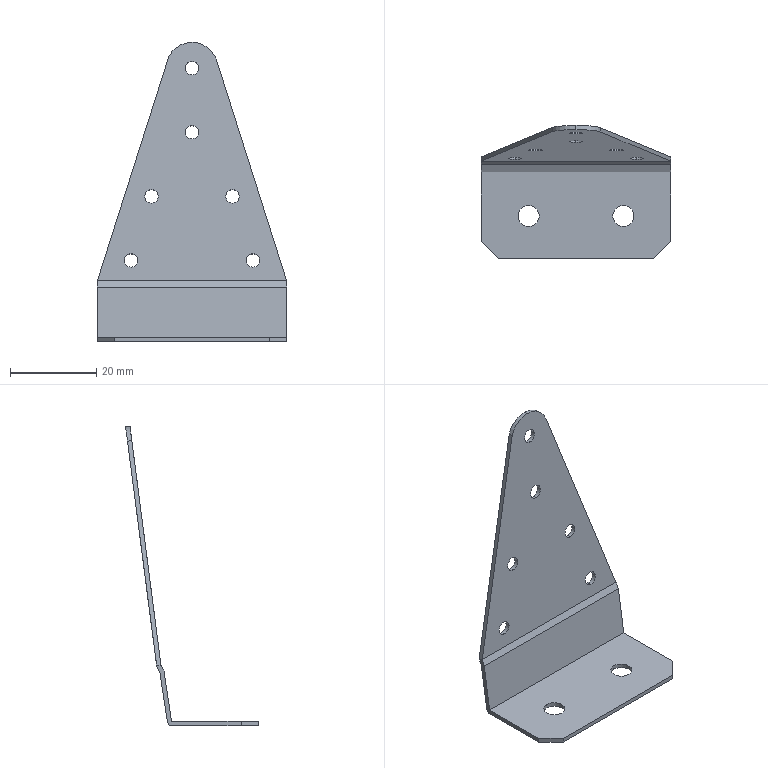Part | SolidWorks | features BaseBody 1 | 1 solid | 34 faces | box 44 x 30.796 x 69.44 mm | volume 2867 mm3 | cylinder 19 | plane 15 | commonest cylinder face diameters 3.2 x12 4.9 x4 12 x2 2 x1
STEP:
#1=CARTESIAN_POINT('',(-153.,101.05,-969.));
#2=VERTEX_POINT('',#1);
#3=CARTESIAN_POINT('',(-153.,105.95,-969.));
#4=VERTEX_POINT('',#3);
#5=CARTESIAN_POINT('',(-153.,103.5,-969.));
#6=DIRECTION('',(0.,0.,-1.));
#7=DIRECTION('',(0.,-1.,0.));
#8=AXIS2_PLACEMENT_3D('',#5,#6,#7);
#9=CIRCLE('',#8,2.45);
#10=EDGE_CURVE('',#2,#4,#9,.T.);
#11=ORIENTED_EDGE('',*,*,#10,.T.);
#12=CARTESIAN_POINT('',(-153.,105.95,-968.));
#13=VERTEX_POINT('',#12);
#14=CARTESIAN_POINT('',(-153.,105.95,-969.));
#15=DIRECTION('',(0.,0.,1.));
#16=VECTOR('',#15,1000.);
#17=LINE('',#14,#16);
#18=EDGE_CURVE('',#4,#13,#17,.T.);
#19=ORIENTED_EDGE('',*,*,#18,.T.);
#20=CARTESIAN_POINT('',(-153.,101.05,-968.));
#21=VERTEX_POINT('',#20);
#22=CARTESIAN_POINT('',(-153.,103.5,-968.));
#23=DIRECTION('',(0.,0.,1.));
#24=DIRECTION('',(0.,-1.,0.));
#25=AXIS2_PLACEMENT_3D('',#22,#23,#24);
#26=CIRCLE('',#25,2.45);
#27=EDGE_CURVE('',#13,#21,#26,.T.);
#28=ORIENTED_EDGE('',*,*,#27,.T.);
#29=CARTESIAN_POINT('',(-153.,101.05,-969.));
#30=DIRECTION('',(0.,0.,1.));
#31=VECTOR('',#30,1000.);
#32=LINE('',#29,#31);
#33=EDGE_CURVE('',#2,#21,#32,.T.);
#34=ORIENTED_EDGE('',*,*,#33,.F.);
#35=EDGE_LOOP('',(#11,#19,#28,#34));
#36=FACE_OUTER_BOUND('',#35,.T.);
#37=CARTESIAN_POINT('',(-153.,103.5,-969.));
#38=DIRECTION('',(0.,0.,1.));
#39=DIRECTION('',(0.,-1.,0.));
#40=AXIS2_PLACEMENT_3D('',#37,#38,#39);
#41=CYLINDRICAL_SURFACE('',#40,2.45);
#42=ADVANCED_FACE('',(#36),#41,.F.);
#43=CARTESIAN_POINT('',(-131.,101.05,-969.));
#44=VERTEX_POINT('',#43);
#45=CARTESIAN_POINT('',(-131.,105.95,-969.));
#46=VERTEX_POINT('',#45);
#47=CARTESIAN_POINT('',(-131.,103.5,-969.));
#48=DIRECTION('',(0.,0.,-1.));
#49=DIRECTION('',(0.,-1.,0.));
#50=AXIS2_PLACEMENT_3D('',#47,#48,#49);
#51=CIRCLE('',#50,2.45);
#52=EDGE_CURVE('',#44,#46,#51,.T.);
#53=ORIENTED_EDGE('',*,*,#52,.T.);
#54=CARTESIAN_POINT('',(-131.,105.95,-968.));
#55=VERTEX_POINT('',#54);
#56=CARTESIAN_POINT('',(-131.,105.95,-969.));
#57=DIRECTION('',(0.,0.,1.));
#58=VECTOR('',#57,1000.);
#59=LINE('',#56,#58);
#60=EDGE_CURVE('',#46,#55,#59,.T.);
#61=ORIENTED_EDGE('',*,*,#60,.T.);
#62=CARTESIAN_POINT('',(-131.,101.05,-968.));
#63=VERTEX_POINT('',#62);
#64=CARTESIAN_POINT('',(-131.,103.5,-968.));
#65=DIRECTION('',(0.,0.,1.));
#66=DIRECTION('',(0.,-1.,0.));
#67=AXIS2_PLACEMENT_3D('',#64,#65,#66);
#68=CIRCLE('',#67,2.45);
#69=EDGE_CURVE('',#55,#63,#68,.T.);
#70=ORIENTED_EDGE('',*,*,#69,.T.);
#71=CARTESIAN_POINT('',(-131.,101.05,-969.));
#72=DIRECTION('',(0.,0.,1.));
#73=VECTOR('',#72,1000.);
#74=LINE('',#71,#73);
#75=EDGE_CURVE('',#44,#63,#74,.T.);
#76=ORIENTED_EDGE('',*,*,#75,.F.);
#77=EDGE_LOOP('',(#53,#61,#70,#76));
#78=FACE_OUTER_BOUND('',#77,.T.);
#79=CARTESIAN_POINT('',(-131.,103.5,-969.));
#80=DIRECTION('',(0.,0.,1.));
#81=DIRECTION('',(0.,-1.,0.));
#82=AXIS2_PLACEMENT_3D('',#79,#80,#81);
#83=CYLINDRICAL_SURFACE('',#82,2.45);
#84=ADVANCED_FACE('',(#78),#83,.F.);
#85=CARTESIAN_POINT('',(-156.144,117.061,-948.549));
#86=VERTEX_POINT('',#85);
#87=CARTESIAN_POINT('',(-156.144,116.649,-951.723));
#88=VERTEX_POINT('',#87);
#89=CARTESIAN_POINT('',(-156.144,116.855,-950.136));
#90=DIRECTION('',(0.,-0.9917,0.1287));
#91=DIRECTION('',(0.,0.1287,0.9917));
#92=AXIS2_PLACEMENT_3D('',#89,#90,#91);
#93=CIRCLE('',#92,1.6);
#94=EDGE_CURVE('',#86,#88,#93,.T.);
#95=ORIENTED_EDGE('',*,*,#94,.T.);
#96=CARTESIAN_POINT('',(-156.144,117.641,-951.851));
#97=VERTEX_POINT('',#96);
#98=CARTESIAN_POINT('',(-156.144,116.649,-951.723));
#99=DIRECTION('',(0.,0.9917,-0.1287));
#100=VECTOR('',#99,1000.);
#101=LINE('',#98,#100);
#102=EDGE_CURVE('',#88,#97,#101,.T.);
#103=ORIENTED_EDGE('',*,*,#102,.T.);
#104=CARTESIAN_POINT('',(-156.144,118.053,-948.678));
#105=VERTEX_POINT('',#104);
#106=CARTESIAN_POINT('',(-156.144,117.847,-950.265));
#107=DIRECTION('',(0.,0.9917,-0.1287));
#108=DIRECTION('',(0.,0.1287,0.9917));
#109=AXIS2_PLACEMENT_3D('',#106,#107,#108);
#110=CIRCLE('',#109,1.6);
#111=EDGE_CURVE('',#97,#105,#110,.T.);
#112=ORIENTED_EDGE('',*,*,#111,.T.);
#113=CARTESIAN_POINT('',(-156.144,117.061,-948.549));
#114=DIRECTION('',(0.,0.9917,-0.1287));
#115=VECTOR('',#114,1000.);
#116=LINE('',#113,#115);
#117=EDGE_CURVE('',#86,#105,#116,.T.);
#118=ORIENTED_EDGE('',*,*,#117,.F.);
#119=EDGE_LOOP('',(#95,#103,#112,#118));
#120=FACE_OUTER_BOUND('',#119,.T.);
#121=CARTESIAN_POINT('',(-156.144,116.855,-950.136));
#122=DIRECTION('',(0.,0.9917,-0.1287));
#123=DIRECTION('',(0.,0.1287,0.9917));
#124=AXIS2_PLACEMENT_3D('',#121,#122,#123);
#125=CYLINDRICAL_SURFACE('',#124,1.6);
#126=ADVANCED_FACE('',(#120),#125,.F.);
#127=CARTESIAN_POINT('',(-151.404,118.991,-933.674));
#128=VERTEX_POINT('',#127);
#129=CARTESIAN_POINT('',(-151.404,118.58,-936.847));
#130=VERTEX_POINT('',#129);
#131=CARTESIAN_POINT('',(-151.404,118.786,-935.261));
#132=DIRECTION('',(0.,-0.9917,0.1287));
#133=DIRECTION('',(0.,0.1287,0.9917));
#134=AXIS2_PLACEMENT_3D('',#131,#132,#133);
#135=CIRCLE('',#134,1.6);
#136=EDGE_CURVE('',#128,#130,#135,.T.);
#137=ORIENTED_EDGE('',*,*,#136,.T.);
#138=CARTESIAN_POINT('',(-151.404,119.571,-936.976));
#139=VERTEX_POINT('',#138);
#140=CARTESIAN_POINT('',(-151.404,118.58,-936.847));
#141=DIRECTION('',(0.,0.9917,-0.1287));
#142=VECTOR('',#141,1000.);
#143=LINE('',#140,#142);
#144=EDGE_CURVE('',#130,#139,#143,.T.);
#145=ORIENTED_EDGE('',*,*,#144,.T.);
#146=CARTESIAN_POINT('',(-151.404,119.983,-933.803));
#147=VERTEX_POINT('',#146);
#148=CARTESIAN_POINT('',(-151.404,119.777,-935.389));
#149=DIRECTION('',(0.,0.9917,-0.1287));
#150=DIRECTION('',(0.,0.1287,0.9917));
#151=AXIS2_PLACEMENT_3D('',#148,#149,#150);
#152=CIRCLE('',#151,1.6);
#153=EDGE_CURVE('',#139,#147,#152,.T.);
#154=ORIENTED_EDGE('',*,*,#153,.T.);
#155=CARTESIAN_POINT('',(-151.404,118.991,-933.674));
#156=DIRECTION('',(0.,0.9917,-0.1287));
#157=VECTOR('',#156,1000.);
#158=LINE('',#155,#157);
#159=EDGE_CURVE('',#128,#147,#158,.T.);
#160=ORIENTED_EDGE('',*,*,#159,.F.);
#161=EDGE_LOOP('',(#137,#145,#154,#160));
#162=FACE_OUTER_BOUND('',#161,.T.);
#163=CARTESIAN_POINT('',(-151.404,118.786,-935.261));
#164=DIRECTION('',(0.,0.9917,-0.1287));
#165=DIRECTION('',(0.,0.1287,0.9917));
#166=AXIS2_PLACEMENT_3D('',#163,#164,#165);
#167=CYLINDRICAL_SURFACE('',#166,1.6);
#168=ADVANCED_FACE('',(#162),#167,.F.);
#169=CARTESIAN_POINT('',(-142.,122.852,-903.924));
#170=VERTEX_POINT('',#169);
#171=CARTESIAN_POINT('',(-142.,122.44,-907.097));
#172=VERTEX_POINT('',#171);
#173=CARTESIAN_POINT('',(-142.,122.646,-905.51));
#174=DIRECTION('',(0.,-0.9917,0.1287));
#175=DIRECTION('',(0.,0.1287,0.9917));
#176=AXIS2_PLACEMENT_3D('',#173,#174,#175);
#177=CIRCLE('',#176,1.6);
#178=EDGE_CURVE('',#170,#172,#177,.T.);
#179=ORIENTED_EDGE('',*,*,#178,.T.);
#180=CARTESIAN_POINT('',(-142.,123.432,-907.226));
#181=VERTEX_POINT('',#180);
#182=CARTESIAN_POINT('',(-142.,122.44,-907.097));
#183=DIRECTION('',(0.,0.9917,-0.1287));
#184=VECTOR('',#183,1000.);
#185=LINE('',#182,#184);
#186=EDGE_CURVE('',#172,#181,#185,.T.);
#187=ORIENTED_EDGE('',*,*,#186,.T.);
#188=CARTESIAN_POINT('',(-142.,123.844,-904.052));
#189=VERTEX_POINT('',#188);
#190=CARTESIAN_POINT('',(-142.,123.638,-905.639));
#191=DIRECTION('',(0.,0.9917,-0.1287));
#192=DIRECTION('',(0.,0.1287,0.9917));
#193=AXIS2_PLACEMENT_3D('',#190,#191,#192);
#194=CIRCLE('',#193,1.6);
#195=EDGE_CURVE('',#181,#189,#194,.T.);
#196=ORIENTED_EDGE('',*,*,#195,.T.);
#197=CARTESIAN_POINT('',(-142.,122.852,-903.924));
#198=DIRECTION('',(0.,0.9917,-0.1287));
#199=VECTOR('',#198,1000.);
#200=LINE('',#197,#199);
#201=EDGE_CURVE('',#170,#189,#200,.T.);
#202=ORIENTED_EDGE('',*,*,#201,.F.);
#203=EDGE_LOOP('',(#179,#187,#196,#202));
#204=FACE_OUTER_BOUND('',#203,.T.);
#205=CARTESIAN_POINT('',(-142.,122.646,-905.51));
#206=DIRECTION('',(0.,0.9917,-0.1287));
#207=DIRECTION('',(0.,0.1287,0.9917));
#208=AXIS2_PLACEMENT_3D('',#205,#206,#207);
#209=CYLINDRICAL_SURFACE('',#208,1.6);
#210=ADVANCED_FACE('',(#204),#209,.F.);
#211=CARTESIAN_POINT('',(-142.,120.922,-918.799));
#212=VERTEX_POINT('',#211);
#213=CARTESIAN_POINT('',(-142.,120.51,-921.972));
#214=VERTEX_POINT('',#213);
#215=CARTESIAN_POINT('',(-142.,120.716,-920.386));
#216=DIRECTION('',(0.,-0.9917,0.1287));
#217=DIRECTION('',(0.,0.1287,0.9917));
#218=AXIS2_PLACEMENT_3D('',#215,#216,#217);
#219=CIRCLE('',#218,1.6);
#220=EDGE_CURVE('',#212,#214,#219,.T.);
#221=ORIENTED_EDGE('',*,*,#220,.T.);
#222=CARTESIAN_POINT('',(-142.,121.502,-922.101));
#223=VERTEX_POINT('',#222);
#224=CARTESIAN_POINT('',(-142.,120.51,-921.972));
#225=DIRECTION('',(0.,0.9917,-0.1287));
#226=VECTOR('',#225,1000.);
#227=LINE('',#224,#226);
#228=EDGE_CURVE('',#214,#223,#227,.T.);
#229=ORIENTED_EDGE('',*,*,#228,.T.);
#230=CARTESIAN_POINT('',(-142.,121.913,-918.928));
#231=VERTEX_POINT('',#230);
#232=CARTESIAN_POINT('',(-142.,121.708,-920.514));
#233=DIRECTION('',(0.,0.9917,-0.1287));
#234=DIRECTION('',(0.,0.1287,0.9917));
#235=AXIS2_PLACEMENT_3D('',#232,#233,#234);
#236=CIRCLE('',#235,1.6);
#237=EDGE_CURVE('',#223,#231,#236,.T.);
#238=ORIENTED_EDGE('',*,*,#237,.T.);
#239=CARTESIAN_POINT('',(-142.,120.922,-918.799));
#240=DIRECTION('',(0.,0.9917,-0.1287));
#241=VECTOR('',#240,1000.);
#242=LINE('',#239,#241);
#243=EDGE_CURVE('',#212,#231,#242,.T.);
#244=ORIENTED_EDGE('',*,*,#243,.F.);
#245=EDGE_LOOP('',(#221,#229,#238,#244));
#246=FACE_OUTER_BOUND('',#245,.T.);
#247=CARTESIAN_POINT('',(-142.,120.716,-920.386));
#248=DIRECTION('',(0.,0.9917,-0.1287));
#249=DIRECTION('',(0.,0.1287,0.9917));
#250=AXIS2_PLACEMENT_3D('',#247,#248,#249);
#251=CYLINDRICAL_SURFACE('',#250,1.6);
#252=ADVANCED_FACE('',(#246),#251,.F.);
#253=CARTESIAN_POINT('',(-132.596,118.991,-933.674));
#254=VERTEX_POINT('',#253);
#255=CARTESIAN_POINT('',(-132.596,118.58,-936.847));
#256=VERTEX_POINT('',#255);
#257=CARTESIAN_POINT('',(-132.596,118.786,-935.261));
#258=DIRECTION('',(0.,-0.9917,0.1287));
#259=DIRECTION('',(0.,0.1287,0.9917));
#260=AXIS2_PLACEMENT_3D('',#257,#258,#259);
#261=CIRCLE('',#260,1.6);
#262=EDGE_CURVE('',#254,#256,#261,.T.);
#263=ORIENTED_EDGE('',*,*,#262,.T.);
#264=CARTESIAN_POINT('',(-132.596,119.571,-936.976));
#265=VERTEX_POINT('',#264);
#266=CARTESIAN_POINT('',(-132.596,118.58,-936.847));
#267=DIRECTION('',(0.,0.9917,-0.1287));
#268=VECTOR('',#267,1000.);
#269=LINE('',#266,#268);
#270=EDGE_CURVE('',#256,#265,#269,.T.);
#271=ORIENTED_EDGE('',*,*,#270,.T.);
#272=CARTESIAN_POINT('',(-132.596,119.983,-933.803));
#273=VERTEX_POINT('',#272);
#274=CARTESIAN_POINT('',(-132.596,119.777,-935.389));
#275=DIRECTION('',(0.,0.9917,-0.1287));
#276=DIRECTION('',(0.,0.1287,0.9917));
#277=AXIS2_PLACEMENT_3D('',#274,#275,#276);
#278=CIRCLE('',#277,1.6);
#279=EDGE_CURVE('',#265,#273,#278,.T.);
#280=ORIENTED_EDGE('',*,*,#279,.T.);
#281=CARTESIAN_POINT('',(-132.596,118.991,-933.674));
#282=DIRECTION('',(0.,0.9917,-0.1287));
#283=VECTOR('',#282,1000.);
#284=LINE('',#281,#283);
#285=EDGE_CURVE('',#254,#273,#284,.T.);
#286=ORIENTED_EDGE('',*,*,#285,.F.);
#287=EDGE_LOOP('',(#263,#271,#280,#286));
#288=FACE_OUTER_BOUND('',#287,.T.);
#289=CARTESIAN_POINT('',(-132.596,118.786,-935.261));
#290=DIRECTION('',(0.,0.9917,-0.1287));
#291=DIRECTION('',(0.,0.1287,0.9917));
#292=AXIS2_PLACEMENT_3D('',#289,#290,#291);
#293=CYLINDRICAL_SURFACE('',#292,1.6);
#294=ADVANCED_FACE('',(#288),#293,.F.);
#295=CARTESIAN_POINT('',(-127.856,117.061,-948.549));
#296=VERTEX_POINT('',#295);
#297=CARTESIAN_POINT('',(-127.856,116.649,-951.723));
#298=VERTEX_POINT('',#297);
#299=CARTESIAN_POINT('',(-127.856,116.855,-950.136));
#300=DIRECTION('',(0.,-0.9917,0.1287));
#301=DIRECTION('',(0.,0.1287,0.9917));
#302=AXIS2_PLACEMENT_3D('',#299,#300,#301);
#303=CIRCLE('',#302,1.6);
#304=EDGE_CURVE('',#296,#298,#303,.T.);
#305=ORIENTED_EDGE('',*,*,#304,.T.);
#306=CARTESIAN_POINT('',(-127.856,117.641,-951.851));
#307=VERTEX_POINT('',#306);
#308=CARTESIAN_POINT('',(-127.856,116.649,-951.723));
#309=DIRECTION('',(0.,0.9917,-0.1287));
#310=VECTOR('',#309,1000.);
#311=LINE('',#308,#310);
#312=EDGE_CURVE('',#298,#307,#311,.T.);
#313=ORIENTED_EDGE('',*,*,#312,.T.);
#314=CARTESIAN_POINT('',(-127.856,118.053,-948.678));
#315=VERTEX_POINT('',#314);
#316=CARTESIAN_POINT('',(-127.856,117.847,-950.265));
#317=DIRECTION('',(0.,0.9917,-0.1287));
#318=DIRECTION('',(0.,0.1287,0.9917));
#319=AXIS2_PLACEMENT_3D('',#316,#317,#318);
#320=CIRCLE('',#319,1.6);
#321=EDGE_CURVE('',#307,#315,#320,.T.);
#322=ORIENTED_EDGE('',*,*,#321,.T.);
#323=CARTESIAN_POINT('',(-127.856,117.061,-948.549));
#324=DIRECTION('',(0.,0.9917,-0.1287));
#325=VECTOR('',#324,1000.);
#326=LINE('',#323,#325);
#327=EDGE_CURVE('',#296,#315,#326,.T.);
#328=ORIENTED_EDGE('',*,*,#327,.F.);
#329=EDGE_LOOP('',(#305,#313,#322,#328));
#330=FACE_OUTER_BOUND('',#329,.T.);
#331=CARTESIAN_POINT('',(-127.856,116.855,-950.136));
#332=DIRECTION('',(0.,0.9917,-0.1287));
#333=DIRECTION('',(0.,0.1287,0.9917));
#334=AXIS2_PLACEMENT_3D('',#331,#332,#333);
#335=CYLINDRICAL_SURFACE('',#334,1.6);
#336=ADVANCED_FACE('',(#330),#335,.F.);
#337=CARTESIAN_POINT('',(-147.37,122.99,-902.856));
#338=VERTEX_POINT('',#337);
#339=CARTESIAN_POINT('',(-142.,123.418,-899.56));
#340=VERTEX_POINT('',#339);
#341=CARTESIAN_POINT('',(-142.,122.646,-905.51));
#342=DIRECTION('',(0.,0.9917,-0.1287));
#343=DIRECTION('',(0.,0.1287,0.9917));
#344=AXIS2_PLACEMENT_3D('',#341,#342,#343);
#345=CIRCLE('',#344,6.);
#346=EDGE_CURVE('',#338,#340,#345,.T.);
#347=ORIENTED_EDGE('',*,*,#346,.T.);
#348=CARTESIAN_POINT('',(-142.,124.41,-899.689));
#349=VERTEX_POINT('',#348);
#350=CARTESIAN_POINT('',(-142.,123.418,-899.56));
#351=DIRECTION('',(0.,0.9917,-0.1287));
#352=VECTOR('',#351,1000.);
#353=LINE('',#350,#352);
#354=EDGE_CURVE('',#340,#349,#353,.T.);
#355=ORIENTED_EDGE('',*,*,#354,.T.);
#356=CARTESIAN_POINT('',(-147.37,123.982,-902.985));
#357=VERTEX_POINT('',#356);
#358=CARTESIAN_POINT('',(-142.,123.638,-905.639));
#359=DIRECTION('',(0.,-0.9917,0.1287));
#360=DIRECTION('',(0.,0.1287,0.9917));
#361=AXIS2_PLACEMENT_3D('',#358,#359,#360);
#362=CIRCLE('',#361,6.);
#363=EDGE_CURVE('',#349,#357,#362,.T.);
#364=ORIENTED_EDGE('',*,*,#363,.T.);
#365=CARTESIAN_POINT('',(-147.37,123.486,-902.921));
#366=DIRECTION('',(0.,0.9917,-0.1287));
#367=VECTOR('',#366,1000.);
#368=LINE('',#365,#367);
#369=EDGE_CURVE('',#338,#357,#368,.T.);
#370=ORIENTED_EDGE('',*,*,#369,.F.);
#371=EDGE_LOOP('',(#347,#355,#364,#370));
#372=FACE_OUTER_BOUND('',#371,.T.);
#373=CARTESIAN_POINT('',(-142.,122.646,-905.51));
#374=DIRECTION('',(0.,0.9917,-0.1287));
#375=DIRECTION('',(0.,0.1287,0.9917));
#376=AXIS2_PLACEMENT_3D('',#373,#374,#375);
#377=CYLINDRICAL_SURFACE('',#376,6.);
#378=ADVANCED_FACE('',(#372),#377,.T.);
#379=ORIENTED_EDGE('',*,*,#18,.F.);
#380=CARTESIAN_POINT('',(-153.,103.5,-969.));
#381=DIRECTION('',(0.,0.,-1.));
#382=DIRECTION('',(0.,-1.,0.));
#383=AXIS2_PLACEMENT_3D('',#380,#381,#382);
#384=CIRCLE('',#383,2.45);
#385=EDGE_CURVE('',#4,#2,#384,.T.);
#386=ORIENTED_EDGE('',*,*,#385,.T.);
#387=ORIENTED_EDGE('',*,*,#33,.T.);
#388=CARTESIAN_POINT('',(-153.,103.5,-968.));
#389=DIRECTION('',(0.,0.,1.));
#390=DIRECTION('',(0.,-1.,0.));
#391=AXIS2_PLACEMENT_3D('',#388,#389,#390);
#392=CIRCLE('',#391,2.45);
#393=EDGE_CURVE('',#21,#13,#392,.T.);
#394=ORIENTED_EDGE('',*,*,#393,.T.);
#395=EDGE_LOOP('',(#379,#386,#387,#394));
#396=FACE_OUTER_BOUND('',#395,.T.);
#397=CARTESIAN_POINT('',(-153.,103.5,-969.));
#398=DIRECTION('',(0.,0.,1.));
#399=DIRECTION('',(0.,-1.,0.));
#400=AXIS2_PLACEMENT_3D('',#397,#398,#399);
#401=CYLINDRICAL_SURFACE('',#400,2.45);
#402=ADVANCED_FACE('',(#396),#401,.F.);
#403=CARTESIAN_POINT('',(-131.,103.5,-968.));
#404=DIRECTION('',(0.,0.,1.));
#405=DIRECTION('',(0.,-1.,0.));
#406=AXIS2_PLACEMENT_3D('',#403,#404,#405);
#407=CIRCLE('',#406,2.45);
#408=EDGE_CURVE('',#63,#55,#407,.T.);
#409=ORIENTED_EDGE('',*,*,#408,.F.);
#410=ORIENTED_EDGE('',*,*,#69,.F.);
#411=EDGE_LOOP('',(#409,#410));
#412=FACE_BOUND('',#411,.T.);
#413=ORIENTED_EDGE('',*,*,#393,.F.);
#414=ORIENTED_EDGE('',*,*,#27,.F.);
#415=EDGE_LOOP('',(#413,#414));
#416=FACE_BOUND('',#415,.T.);
#417=CARTESIAN_POINT('',(-160.,93.614,-968.));
#418=VERTEX_POINT('',#417);
#419=CARTESIAN_POINT('',(-164.,97.614,-968.));
#420=VERTEX_POINT('',#419);
#421=CARTESIAN_POINT('',(-164.,97.614,-968.));
#422=DIRECTION('',(-0.7071,0.7071,0.));
#423=VECTOR('',#422,1000.);
#424=LINE('',#421,#423);
#425=EDGE_CURVE('',#418,#420,#424,.T.);
#426=ORIENTED_EDGE('',*,*,#425,.F.);
#427=CARTESIAN_POINT('',(-124.,93.614,-968.));
#428=VERTEX_POINT('',#427);
#429=CARTESIAN_POINT('',(-142.,93.614,-968.));
#430=DIRECTION('',(-1.,0.,0.));
#431=VECTOR('',#430,1000.);
#432=LINE('',#429,#431);
#433=EDGE_CURVE('',#428,#418,#432,.T.);
#434=ORIENTED_EDGE('',*,*,#433,.F.);
#435=CARTESIAN_POINT('',(-120.,97.614,-968.));
#436=VERTEX_POINT('',#435);
#437=CARTESIAN_POINT('',(-124.,93.614,-968.));
#438=DIRECTION('',(-0.7071,-0.7071,0.));
#439=VECTOR('',#438,1000.);
#440=LINE('',#437,#439);
#441=EDGE_CURVE('',#436,#428,#440,.T.);
#442=ORIENTED_EDGE('',*,*,#441,.F.);
#443=CARTESIAN_POINT('',(-120.,113.753,-968.));
#444=VERTEX_POINT('',#443);
#445=CARTESIAN_POINT('',(-120.,103.684,-968.));
#446=DIRECTION('',(0.,-1.,0.));
#447=VECTOR('',#446,1000.);
#448=LINE('',#445,#447);
#449=EDGE_CURVE('',#444,#436,#448,.T.);
#450=ORIENTED_EDGE('',*,*,#449,.F.);
#451=CARTESIAN_POINT('',(-164.,113.753,-968.));
#452=VERTEX_POINT('',#451);
#453=CARTESIAN_POINT('',(-142.,113.753,-968.));
#454=DIRECTION('',(1.,0.,0.));
#455=VECTOR('',#454,1000.);
#456=LINE('',#453,#455);
#457=EDGE_CURVE('',#452,#444,#456,.T.);
#458=ORIENTED_EDGE('',*,*,#457,.F.);
#459=CARTESIAN_POINT('',(-164.,103.684,-968.));
#460=DIRECTION('',(0.,1.,0.));
#461=VECTOR('',#460,1000.);
#462=LINE('',#459,#461);
#463=EDGE_CURVE('',#420,#452,#462,.T.);
#464=ORIENTED_EDGE('',*,*,#463,.F.);
#465=EDGE_LOOP('',(#426,#434,#442,#450,#458,#464));
#466=FACE_OUTER_BOUND('',#465,.T.);
#467=CARTESIAN_POINT('',(-120.,93.614,-968.));
#468=DIRECTION('',(0.,0.,-1.));
#469=DIRECTION('',(-1.,0.,0.));
#470=AXIS2_PLACEMENT_3D('',#467,#468,#469);
#471=PLANE('',#470);
#472=ADVANCED_FACE('',(#412,#416,#466),#471,.F.);
#473=ORIENTED_EDGE('',*,*,#52,.F.);
#474=CARTESIAN_POINT('',(-131.,103.5,-969.));
#475=DIRECTION('',(0.,0.,-1.));
#476=DIRECTION('',(0.,-1.,0.));
#477=AXIS2_PLACEMENT_3D('',#474,#475,#476);
#478=CIRCLE('',#477,2.45);
#479=EDGE_CURVE('',#46,#44,#478,.T.);
#480=ORIENTED_EDGE('',*,*,#479,.F.);
#481=EDGE_LOOP('',(#473,#480));
#482=FACE_BOUND('',#481,.T.);
#483=ORIENTED_EDGE('',*,*,#10,.F.);
#484=ORIENTED_EDGE('',*,*,#385,.F.);
#485=EDGE_LOOP('',(#483,#484));
#486=FACE_BOUND('',#485,.T.);
#487=CARTESIAN_POINT('',(-164.,97.614,-969.));
#488=VERTEX_POINT('',#487);
#489=CARTESIAN_POINT('',(-160.,93.614,-969.));
#490=VERTEX_POINT('',#489);
#491=CARTESIAN_POINT('',(-164.,97.614,-969.));
#492=DIRECTION('',(0.7071,-0.7071,0.));
#493=VECTOR('',#492,1000.);
#494=LINE('',#491,#493);
#495=EDGE_CURVE('',#488,#490,#494,.T.);
#496=ORIENTED_EDGE('',*,*,#495,.F.);
#497=CARTESIAN_POINT('',(-164.,113.753,-969.));
#498=VERTEX_POINT('',#497);
#499=CARTESIAN_POINT('',(-164.,103.684,-969.));
#500=DIRECTION('',(0.,-1.,0.));
#501=VECTOR('',#500,1000.);
#502=LINE('',#499,#501);
#503=EDGE_CURVE('',#498,#488,#502,.T.);
#504=ORIENTED_EDGE('',*,*,#503,.F.);
#505=CARTESIAN_POINT('',(-120.,113.753,-969.));
#506=VERTEX_POINT('',#505);
#507=CARTESIAN_POINT('',(-142.,113.753,-969.));
#508=DIRECTION('',(-1.,0.,0.));
#509=VECTOR('',#508,1000.);
#510=LINE('',#507,#509);
#511=EDGE_CURVE('',#506,#498,#510,.T.);
#512=ORIENTED_EDGE('',*,*,#511,.F.);
#513=CARTESIAN_POINT('',(-120.,97.614,-969.));
#514=VERTEX_POINT('',#513);
#515=CARTESIAN_POINT('',(-120.,103.684,-969.));
#516=DIRECTION('',(0.,1.,0.));
#517=VECTOR('',#516,1000.);
#518=LINE('',#515,#517);
#519=EDGE_CURVE('',#514,#506,#518,.T.);
#520=ORIENTED_EDGE('',*,*,#519,.F.);
#521=CARTESIAN_POINT('',(-124.,93.614,-969.));
#522=VERTEX_POINT('',#521);
#523=CARTESIAN_POINT('',(-124.,93.614,-969.));
#524=DIRECTION('',(0.7071,0.7071,0.));
#525=VECTOR('',#524,1000.);
#526=LINE('',#523,#525);
#527=EDGE_CURVE('',#522,#514,#526,.T.);
#528=ORIENTED_EDGE('',*,*,#527,.F.);
#529=CARTESIAN_POINT('',(-142.,93.614,-969.));
#530=DIRECTION('',(1.,0.,0.));
#531=VECTOR('',#530,1000.);
#532=LINE('',#529,#531);
#533=EDGE_CURVE('',#490,#522,#532,.T.);
#534=ORIENTED_EDGE('',*,*,#533,.F.);
#535=EDGE_LOOP('',(#496,#504,#512,#520,#528,#534));
#536=FACE_OUTER_BOUND('',#535,.T.);
#537=CARTESIAN_POINT('',(-164.,93.614,-969.));
#538=DIRECTION('',(0.,0.,1.));
#539=DIRECTION('',(1.,0.,0.));
#540=AXIS2_PLACEMENT_3D('',#537,#538,#539);
#541=PLANE('',#540);
#542=ADVANCED_FACE('',(#482,#486,#536),#541,.F.);
#543=ORIENTED_EDGE('',*,*,#60,.F.);
#544=ORIENTED_EDGE('',*,*,#479,.T.);
#545=ORIENTED_EDGE('',*,*,#75,.T.);
#546=ORIENTED_EDGE('',*,*,#408,.T.);
#547=EDGE_LOOP('',(#543,#544,#545,#546));
#548=FACE_OUTER_BOUND('',#547,.T.);
#549=CARTESIAN_POINT('',(-131.,103.5,-969.));
#550=DIRECTION('',(0.,0.,1.));
#551=DIRECTION('',(0.,-1.,0.));
#552=AXIS2_PLACEMENT_3D('',#549,#550,#551);
#553=CYLINDRICAL_SURFACE('',#552,2.45);
#554=ADVANCED_FACE('',(#548),#553,.F.);
#555=CARTESIAN_POINT('',(-164.,116.471,-956.644));
#556=VERTEX_POINT('',#555);
#557=CARTESIAN_POINT('',(-164.,114.742,-968.149));
#558=VERTEX_POINT('',#557);
#559=CARTESIAN_POINT('',(-164.,116.471,-956.644));
#560=DIRECTION('',(0.,-0.1486,-0.9889));
#561=VECTOR('',#560,1000.);
#562=LINE('',#559,#561);
#563=EDGE_CURVE('',#556,#558,#562,.T.);
#564=ORIENTED_EDGE('',*,*,#563,.T.);
#565=CARTESIAN_POINT('',(-164.,113.753,-968.));
#566=DIRECTION('',(-1.,0.,0.));
#567=DIRECTION('',(0.,0.,-1.));
#568=AXIS2_PLACEMENT_3D('',#565,#566,#567);
#569=CIRCLE('',#568,1.);
#570=EDGE_CURVE('',#558,#498,#569,.T.);
#571=ORIENTED_EDGE('',*,*,#570,.T.);
#572=ORIENTED_EDGE('',*,*,#503,.T.);
#573=CARTESIAN_POINT('',(-164.,97.614,-961.976));
#574=DIRECTION('',(0.,0.,1.));
#575=VECTOR('',#574,1000.);
#576=LINE('',#573,#575);
#577=EDGE_CURVE('',#488,#420,#576,.T.);
#578=ORIENTED_EDGE('',*,*,#577,.T.);
#579=ORIENTED_EDGE('',*,*,#463,.T.);
#580=CARTESIAN_POINT('',(-164.,115.506,-956.337));
#581=VERTEX_POINT('',#580);
#582=CARTESIAN_POINT('',(-164.,113.753,-968.));
#583=DIRECTION('',(0.,0.1486,0.9889));
#584=VECTOR('',#583,1000.);
#585=LINE('',#582,#584);
#586=EDGE_CURVE('',#452,#581,#585,.T.);
#587=ORIENTED_EDGE('',*,*,#586,.T.);
#588=CARTESIAN_POINT('',(-164.,116.16,-955.035));
#589=VERTEX_POINT('',#588);
#590=CARTESIAN_POINT('',(-164.,115.873,-955.606));
#591=DIRECTION('',(0.,0.4487,0.8937));
#592=VECTOR('',#591,1000.);
#593=LINE('',#590,#592);
#594=EDGE_CURVE('',#581,#589,#593,.T.);
#595=ORIENTED_EDGE('',*,*,#594,.T.);
#596=CARTESIAN_POINT('',(-164.,117.21,-955.172));
#597=VERTEX_POINT('',#596);
#598=CARTESIAN_POINT('',(-164.,116.16,-955.035));
#599=DIRECTION('',(0.,0.9917,-0.1287));
#600=VECTOR('',#599,1000.);
#601=LINE('',#598,#600);
#602=EDGE_CURVE('',#589,#597,#601,.T.);
#603=ORIENTED_EDGE('',*,*,#602,.T.);
#604=CARTESIAN_POINT('',(-164.,116.841,-955.908));
#605=DIRECTION('',(0.,-0.4487,-0.8937));
#606=VECTOR('',#605,1000.);
#607=LINE('',#604,#606);
#608=EDGE_CURVE('',#597,#556,#607,.T.);
#609=ORIENTED_EDGE('',*,*,#608,.T.);
#610=EDGE_LOOP('',(#564,#571,#572,#578,#579,#587,#595,#603,#609));
#611=FACE_OUTER_BOUND('',#610,.T.);
#612=CARTESIAN_POINT('',(-164.,97.614,-969.));
#613=DIRECTION('',(-1.,0.,0.));
#614=DIRECTION('',(0.,0.,1.));
#615=AXIS2_PLACEMENT_3D('',#612,#613,#614);
#616=PLANE('',#615);
#617=ADVANCED_FACE('',(#611),#616,.T.);
#618=ORIENTED_EDGE('',*,*,#425,.T.);
#619=ORIENTED_EDGE('',*,*,#577,.F.);
#620=ORIENTED_EDGE('',*,*,#495,.T.);
#621=CARTESIAN_POINT('',(-160.,93.614,-968.5));
#622=DIRECTION('',(0.,0.,1.));
#623=VECTOR('',#622,1000.);
#624=LINE('',#621,#623);
#625=EDGE_CURVE('',#490,#418,#624,.T.);
#626=ORIENTED_EDGE('',*,*,#625,.T.);
#627=EDGE_LOOP('',(#618,#619,#620,#626));
#628=FACE_OUTER_BOUND('',#627,.T.);
#629=CARTESIAN_POINT('',(-164.,97.614,-968.));
#630=DIRECTION('',(-0.7071,-0.7071,0.));
#631=DIRECTION('',(0.,0.,-1.));
#632=AXIS2_PLACEMENT_3D('',#629,#630,#631);
#633=PLANE('',#632);
#634=ADVANCED_FACE('',(#628),#633,.T.);
#635=ORIENTED_EDGE('',*,*,#625,.F.);
#636=ORIENTED_EDGE('',*,*,#533,.T.);
#637=CARTESIAN_POINT('',(-124.,93.614,-968.5));
#638=DIRECTION('',(0.,0.,-1.));
#639=VECTOR('',#638,1000.);
#640=LINE('',#637,#639);
#641=EDGE_CURVE('',#428,#522,#640,.T.);
#642=ORIENTED_EDGE('',*,*,#641,.F.);
#643=ORIENTED_EDGE('',*,*,#433,.T.);
#644=EDGE_LOOP('',(#635,#636,#642,#643));
#645=FACE_OUTER_BOUND('',#644,.T.);
#646=CARTESIAN_POINT('',(-160.,93.614,-969.));
#647=DIRECTION('',(0.,1.,0.));
#648=DIRECTION('',(0.,0.,1.));
#649=AXIS2_PLACEMENT_3D('',#646,#647,#648);
#650=PLANE('',#649);
#651=ADVANCED_FACE('',(#645),#650,.F.);
#652=CARTESIAN_POINT('',(-120.,97.614,-968.5));
#653=DIRECTION('',(0.,0.,-1.));
#654=VECTOR('',#653,1000.);
#655=LINE('',#652,#654);
#656=EDGE_CURVE('',#436,#514,#655,.T.);
#657=ORIENTED_EDGE('',*,*,#656,.F.);
#658=ORIENTED_EDGE('',*,*,#441,.T.);
#659=ORIENTED_EDGE('',*,*,#641,.T.);
#660=ORIENTED_EDGE('',*,*,#527,.T.);
#661=EDGE_LOOP('',(#657,#658,#659,#660));
#662=FACE_OUTER_BOUND('',#661,.T.);
#663=CARTESIAN_POINT('',(-124.,93.614,-969.));
#664=DIRECTION('',(-0.7071,0.7071,0.));
#665=DIRECTION('',(0.,0.,1.));
#666=AXIS2_PLACEMENT_3D('',#663,#664,#665);
#667=PLANE('',#666);
#668=ADVANCED_FACE('',(#662),#667,.F.);
#669=ORIENTED_EDGE('',*,*,#656,.T.);
#670=ORIENTED_EDGE('',*,*,#519,.T.);
#671=CARTESIAN_POINT('',(-120.,114.742,-968.149));
#672=VERTEX_POINT('',#671);
#673=CARTESIAN_POINT('',(-120.,113.753,-968.));
#674=DIRECTION('',(-1.,0.,0.));
#675=DIRECTION('',(0.,0.,-1.));
#676=AXIS2_PLACEMENT_3D('',#673,#674,#675);
#677=CIRCLE('',#676,1.);
#678=EDGE_CURVE('',#672,#506,#677,.T.);
#679=ORIENTED_EDGE('',*,*,#678,.F.);
#680=CARTESIAN_POINT('',(-120.,116.471,-956.644));
#681=VERTEX_POINT('',#680);
#682=CARTESIAN_POINT('',(-120.,116.471,-956.644));
#683=DIRECTION('',(0.,-0.1486,-0.9889));
#684=VECTOR('',#683,1000.);
#685=LINE('',#682,#684);
#686=EDGE_CURVE('',#681,#672,#685,.T.);
#687=ORIENTED_EDGE('',*,*,#686,.F.);
#688=CARTESIAN_POINT('',(-120.,117.21,-955.172));
#689=VERTEX_POINT('',#688);
#690=CARTESIAN_POINT('',(-120.,116.841,-955.908));
#691=DIRECTION('',(0.,0.4487,0.8937));
#692=VECTOR('',#691,1000.);
#693=LINE('',#690,#692);
#694=EDGE_CURVE('',#681,#689,#693,.T.);
#695=ORIENTED_EDGE('',*,*,#694,.T.);
#696=CARTESIAN_POINT('',(-120.,116.16,-955.035));
#697=VERTEX_POINT('',#696);
#698=CARTESIAN_POINT('',(-120.,117.21,-955.172));
#699=DIRECTION('',(0.,-0.9917,0.1287));
#700=VECTOR('',#699,1000.);
#701=LINE('',#698,#700);
#702=EDGE_CURVE('',#689,#697,#701,.T.);
#703=ORIENTED_EDGE('',*,*,#702,.T.);
#704=CARTESIAN_POINT('',(-120.,115.506,-956.337));
#705=VERTEX_POINT('',#704);
#706=CARTESIAN_POINT('',(-120.,115.873,-955.606));
#707=DIRECTION('',(0.,-0.4487,-0.8937));
#708=VECTOR('',#707,1000.);
#709=LINE('',#706,#708);
#710=EDGE_CURVE('',#697,#705,#709,.T.);
#711=ORIENTED_EDGE('',*,*,#710,.T.);
#712=CARTESIAN_POINT('',(-120.,113.753,-968.));
#713=DIRECTION('',(0.,0.1486,0.9889));
#714=VECTOR('',#713,1000.);
#715=LINE('',#712,#714);
#716=EDGE_CURVE('',#444,#705,#715,.T.);
#717=ORIENTED_EDGE('',*,*,#716,.F.);
#718=ORIENTED_EDGE('',*,*,#449,.T.);
#719=EDGE_LOOP('',(#669,#670,#679,#687,#695,#703,#711,#717,#718));
#720=FACE_OUTER_BOUND('',#719,.T.);
#721=CARTESIAN_POINT('',(-120.,97.614,-969.));
#722=DIRECTION('',(-1.,0.,0.));
#723=DIRECTION('',(0.,0.,1.));
#724=AXIS2_PLACEMENT_3D('',#721,#722,#723);
#725=PLANE('',#724);
#726=ADVANCED_FACE('',(#720),#725,.F.);
#727=CARTESIAN_POINT('',(-142.,115.506,-956.337));
#728=DIRECTION('',(1.,0.,0.));
#729=VECTOR('',#728,1000.);
#730=LINE('',#727,#729);
#731=EDGE_CURVE('',#581,#705,#730,.T.);
#732=ORIENTED_EDGE('',*,*,#731,.F.);
#733=ORIENTED_EDGE('',*,*,#586,.F.);
#734=ORIENTED_EDGE('',*,*,#457,.T.);
#735=ORIENTED_EDGE('',*,*,#716,.T.);
#736=EDGE_LOOP('',(#732,#733,#734,#735));
#737=FACE_OUTER_BOUND('',#736,.T.);
#738=CARTESIAN_POINT('',(-164.,113.753,-968.));
#739=DIRECTION('',(0.,0.9889,-0.1486));
#740=DIRECTION('',(0.,0.1486,0.9889));
#741=AXIS2_PLACEMENT_3D('',#738,#739,#740);
#742=PLANE('',#741);
#743=ADVANCED_FACE('',(#737),#742,.F.);
#744=ORIENTED_EDGE('',*,*,#511,.T.);
#745=ORIENTED_EDGE('',*,*,#570,.F.);
#746=CARTESIAN_POINT('',(-142.,114.742,-968.149));
#747=DIRECTION('',(-1.,0.,0.));
#748=VECTOR('',#747,1000.);
#749=LINE('',#746,#748);
#750=EDGE_CURVE('',#672,#558,#749,.T.);
#751=ORIENTED_EDGE('',*,*,#750,.F.);
#752=ORIENTED_EDGE('',*,*,#678,.T.);
#753=EDGE_LOOP('',(#744,#745,#751,#752));
#754=FACE_OUTER_BOUND('',#753,.T.);
#755=CARTESIAN_POINT('',(-164.,113.753,-968.));
#756=DIRECTION('',(1.,0.,0.));
#757=DIRECTION('',(0.,0.,-1.));
#758=AXIS2_PLACEMENT_3D('',#755,#756,#757);
#759=CYLINDRICAL_SURFACE('',#758,1.);
#760=ADVANCED_FACE('',(#754),#759,.T.);
#761=ORIENTED_EDGE('',*,*,#750,.T.);
#762=ORIENTED_EDGE('',*,*,#563,.F.);
#763=CARTESIAN_POINT('',(-142.,116.471,-956.644));
#764=DIRECTION('',(-1.,0.,0.));
#765=VECTOR('',#764,1000.);
#766=LINE('',#763,#765);
#767=EDGE_CURVE('',#681,#556,#766,.T.);
#768=ORIENTED_EDGE('',*,*,#767,.F.);
#769=ORIENTED_EDGE('',*,*,#686,.T.);
#770=EDGE_LOOP('',(#761,#762,#768,#769));
#771=FACE_OUTER_BOUND('',#770,.T.);
#772=CARTESIAN_POINT('',(-164.,116.471,-956.644));
#773=DIRECTION('',(0.,-0.9889,0.1486));
#774=DIRECTION('',(0.,-0.1486,-0.9889));
#775=AXIS2_PLACEMENT_3D('',#772,#773,#774);
#776=PLANE('',#775);
#777=ADVANCED_FACE('',(#771),#776,.F.);
#778=CARTESIAN_POINT('',(-163.946,116.24,-954.875));
#779=VERTEX_POINT('',#778);
#780=CARTESIAN_POINT('',(-163.946,116.24,-954.875));
#781=DIRECTION('',(-0.2859,-0.43,-0.8564));
#782=VECTOR('',#781,1000.);
#783=LINE('',#780,#782);
#784=EDGE_CURVE('',#779,#589,#783,.T.);
#785=ORIENTED_EDGE('',*,*,#784,.T.);
#786=ORIENTED_EDGE('',*,*,#594,.F.);
#787=ORIENTED_EDGE('',*,*,#731,.T.);
#788=ORIENTED_EDGE('',*,*,#710,.F.);
#789=CARTESIAN_POINT('',(-120.053,116.24,-954.875));
#790=VERTEX_POINT('',#789);
#791=CARTESIAN_POINT('',(-120.,116.16,-955.035));
#792=DIRECTION('',(-0.2846,0.4301,0.8567));
#793=VECTOR('',#792,1000.);
#794=LINE('',#791,#793);
#795=EDGE_CURVE('',#697,#790,#794,.T.);
#796=ORIENTED_EDGE('',*,*,#795,.T.);
#797=CARTESIAN_POINT('',(-142.,116.24,-954.875));
#798=DIRECTION('',(1.,0.,0.));
#799=VECTOR('',#798,1000.);
#800=LINE('',#797,#799);
#801=EDGE_CURVE('',#779,#790,#800,.T.);
#802=ORIENTED_EDGE('',*,*,#801,.F.);
#803=EDGE_LOOP('',(#785,#786,#787,#788,#796,#802));
#804=FACE_OUTER_BOUND('',#803,.T.);
#805=CARTESIAN_POINT('',(-164.,115.506,-956.337));
#806=DIRECTION('',(0.,0.8937,-0.4487));
#807=DIRECTION('',(0.,0.4487,0.8937));
#808=AXIS2_PLACEMENT_3D('',#805,#806,#807);
#809=PLANE('',#808);
#810=ADVANCED_FACE('',(#804),#809,.F.);
#811=ORIENTED_EDGE('',*,*,#767,.T.);
#812=ORIENTED_EDGE('',*,*,#608,.F.);
#813=CARTESIAN_POINT('',(-142.,117.21,-955.172));
#814=DIRECTION('',(-1.,0.,0.));
#815=VECTOR('',#814,1000.);
#816=LINE('',#813,#815);
#817=EDGE_CURVE('',#689,#597,#816,.T.);
#818=ORIENTED_EDGE('',*,*,#817,.F.);
#819=ORIENTED_EDGE('',*,*,#694,.F.);
#820=EDGE_LOOP('',(#811,#812,#818,#819));
#821=FACE_OUTER_BOUND('',#820,.T.);
#822=CARTESIAN_POINT('',(-164.,117.21,-955.172));
#823=DIRECTION('',(0.,-0.8937,0.4487));
#824=DIRECTION('',(0.,-0.4487,-0.8937));
#825=AXIS2_PLACEMENT_3D('',#822,#823,#824);
#826=PLANE('',#825);
#827=ADVANCED_FACE('',(#821),#826,.F.);
#828=ORIENTED_EDGE('',*,*,#94,.F.);
#829=CARTESIAN_POINT('',(-156.144,116.855,-950.136));
#830=DIRECTION('',(0.,-0.9917,0.1287));
#831=DIRECTION('',(0.,0.1287,0.9917));
#832=AXIS2_PLACEMENT_3D('',#829,#830,#831);
#833=CIRCLE('',#832,1.6);
#834=EDGE_CURVE('',#88,#86,#833,.T.);
#835=ORIENTED_EDGE('',*,*,#834,.F.);
#836=EDGE_LOOP('',(#828,#835));
#837=FACE_BOUND('',#836,.T.);
#838=ORIENTED_EDGE('',*,*,#136,.F.);
#839=CARTESIAN_POINT('',(-151.404,118.786,-935.261));
#840=DIRECTION('',(0.,-0.9917,0.1287));
#841=DIRECTION('',(0.,0.1287,0.9917));
#842=AXIS2_PLACEMENT_3D('',#839,#840,#841);
#843=CIRCLE('',#842,1.6);
#844=EDGE_CURVE('',#130,#128,#843,.T.);
#845=ORIENTED_EDGE('',*,*,#844,.F.);
#846=EDGE_LOOP('',(#838,#845));
#847=FACE_BOUND('',#846,.T.);
#848=ORIENTED_EDGE('',*,*,#178,.F.);
#849=CARTESIAN_POINT('',(-142.,122.646,-905.51));
#850=DIRECTION('',(0.,-0.9917,0.1287));
#851=DIRECTION('',(0.,0.1287,0.9917));
#852=AXIS2_PLACEMENT_3D('',#849,#850,#851);
#853=CIRCLE('',#852,1.6);
#854=EDGE_CURVE('',#172,#170,#853,.T.);
#855=ORIENTED_EDGE('',*,*,#854,.F.);
#856=EDGE_LOOP('',(#848,#855));
#857=FACE_BOUND('',#856,.T.);
#858=ORIENTED_EDGE('',*,*,#220,.F.);
#859=CARTESIAN_POINT('',(-142.,120.716,-920.386));
#860=DIRECTION('',(0.,-0.9917,0.1287));
#861=DIRECTION('',(0.,0.1287,0.9917));
#862=AXIS2_PLACEMENT_3D('',#859,#860,#861);
#863=CIRCLE('',#862,1.6);
#864=EDGE_CURVE('',#214,#212,#863,.T.);
#865=ORIENTED_EDGE('',*,*,#864,.F.);
#866=EDGE_LOOP('',(#858,#865));
#867=FACE_BOUND('',#866,.T.);
#868=ORIENTED_EDGE('',*,*,#262,.F.);
#869=CARTESIAN_POINT('',(-132.596,118.786,-935.261));
#870=DIRECTION('',(0.,-0.9917,0.1287));
#871=DIRECTION('',(0.,0.1287,0.9917));
#872=AXIS2_PLACEMENT_3D('',#869,#870,#871);
#873=CIRCLE('',#872,1.6);
#874=EDGE_CURVE('',#256,#254,#873,.T.);
#875=ORIENTED_EDGE('',*,*,#874,.F.);
#876=EDGE_LOOP('',(#868,#875));
#877=FACE_BOUND('',#876,.T.);
#878=ORIENTED_EDGE('',*,*,#304,.F.);
#879=CARTESIAN_POINT('',(-127.856,116.855,-950.136));
#880=DIRECTION('',(0.,-0.9917,0.1287));
#881=DIRECTION('',(0.,0.1287,0.9917));
#882=AXIS2_PLACEMENT_3D('',#879,#880,#881);
#883=CIRCLE('',#882,1.6);
#884=EDGE_CURVE('',#298,#296,#883,.T.);
#885=ORIENTED_EDGE('',*,*,#884,.F.);
#886=EDGE_LOOP('',(#878,#885));
#887=FACE_BOUND('',#886,.T.);
#888=ORIENTED_EDGE('',*,*,#346,.F.);
#889=CARTESIAN_POINT('',(-163.946,116.24,-954.875));
#890=DIRECTION('',(0.3013,0.1227,0.9456));
#891=VECTOR('',#890,1000.);
#892=LINE('',#889,#891);
#893=EDGE_CURVE('',#779,#338,#892,.T.);
#894=ORIENTED_EDGE('',*,*,#893,.F.);
#895=ORIENTED_EDGE('',*,*,#801,.T.);
#896=CARTESIAN_POINT('',(-136.276,122.878,-903.725));
#897=VERTEX_POINT('',#896);
#898=CARTESIAN_POINT('',(-136.276,122.878,-903.725));
#899=DIRECTION('',(0.3,-0.1228,-0.946));
#900=VECTOR('',#899,1000.);
#901=LINE('',#898,#900);
#902=EDGE_CURVE('',#897,#790,#901,.T.);
#903=ORIENTED_EDGE('',*,*,#902,.F.);
#904=CARTESIAN_POINT('',(-142.,122.646,-905.51));
#905=DIRECTION('',(0.,0.9917,-0.1287));
#906=DIRECTION('',(0.,0.1287,0.9917));
#907=AXIS2_PLACEMENT_3D('',#904,#905,#906);
#908=CIRCLE('',#907,6.);
#909=EDGE_CURVE('',#340,#897,#908,.T.);
#910=ORIENTED_EDGE('',*,*,#909,.F.);
#911=EDGE_LOOP('',(#888,#894,#895,#903,#910));
#912=FACE_OUTER_BOUND('',#911,.T.);
#913=CARTESIAN_POINT('',(-164.21,116.24,-954.875));
#914=DIRECTION('',(0.,0.9917,-0.1287));
#915=DIRECTION('',(0.,0.1287,0.9917));
#916=AXIS2_PLACEMENT_3D('',#913,#914,#915);
#917=PLANE('',#916);
#918=ADVANCED_FACE('',(#837,#847,#857,#867,#877,#887,#912),#917,.F.);
#919=CARTESIAN_POINT('',(-156.144,117.847,-950.265));
#920=DIRECTION('',(0.,0.9917,-0.1287));
#921=DIRECTION('',(0.,0.1287,0.9917));
#922=AXIS2_PLACEMENT_3D('',#919,#920,#921);
#923=CIRCLE('',#922,1.6);
#924=EDGE_CURVE('',#105,#97,#923,.T.);
#925=ORIENTED_EDGE('',*,*,#924,.F.);
#926=ORIENTED_EDGE('',*,*,#111,.F.);
#927=EDGE_LOOP('',(#925,#926));
#928=FACE_BOUND('',#927,.T.);
#929=CARTESIAN_POINT('',(-151.404,119.777,-935.389));
#930=DIRECTION('',(0.,0.9917,-0.1287));
#931=DIRECTION('',(0.,0.1287,0.9917));
#932=AXIS2_PLACEMENT_3D('',#929,#930,#931);
#933=CIRCLE('',#932,1.6);
#934=EDGE_CURVE('',#147,#139,#933,.T.);
#935=ORIENTED_EDGE('',*,*,#934,.F.);
#936=ORIENTED_EDGE('',*,*,#153,.F.);
#937=EDGE_LOOP('',(#935,#936));
#938=FACE_BOUND('',#937,.T.);
#939=CARTESIAN_POINT('',(-142.,123.638,-905.639));
#940=DIRECTION('',(0.,0.9917,-0.1287));
#941=DIRECTION('',(0.,0.1287,0.9917));
#942=AXIS2_PLACEMENT_3D('',#939,#940,#941);
#943=CIRCLE('',#942,1.6);
#944=EDGE_CURVE('',#189,#181,#943,.T.);
#945=ORIENTED_EDGE('',*,*,#944,.F.);
#946=ORIENTED_EDGE('',*,*,#195,.F.);
#947=EDGE_LOOP('',(#945,#946));
#948=FACE_BOUND('',#947,.T.);
#949=CARTESIAN_POINT('',(-142.,121.708,-920.514));
#950=DIRECTION('',(0.,0.9917,-0.1287));
#951=DIRECTION('',(0.,0.1287,0.9917));
#952=AXIS2_PLACEMENT_3D('',#949,#950,#951);
#953=CIRCLE('',#952,1.6);
#954=EDGE_CURVE('',#231,#223,#953,.T.);
#955=ORIENTED_EDGE('',*,*,#954,.F.);
#956=ORIENTED_EDGE('',*,*,#237,.F.);
#957=EDGE_LOOP('',(#955,#956));
#958=FACE_BOUND('',#957,.T.);
#959=CARTESIAN_POINT('',(-132.596,119.777,-935.389));
#960=DIRECTION('',(0.,0.9917,-0.1287));
#961=DIRECTION('',(0.,0.1287,0.9917));
#962=AXIS2_PLACEMENT_3D('',#959,#960,#961);
#963=CIRCLE('',#962,1.6);
#964=EDGE_CURVE('',#273,#265,#963,.T.);
#965=ORIENTED_EDGE('',*,*,#964,.F.);
#966=ORIENTED_EDGE('',*,*,#279,.F.);
#967=EDGE_LOOP('',(#965,#966));
#968=FACE_BOUND('',#967,.T.);
#969=CARTESIAN_POINT('',(-127.856,117.847,-950.265));
#970=DIRECTION('',(0.,0.9917,-0.1287));
#971=DIRECTION('',(0.,0.1287,0.9917));
#972=AXIS2_PLACEMENT_3D('',#969,#970,#971);
#973=CIRCLE('',#972,1.6);
#974=EDGE_CURVE('',#315,#307,#973,.T.);
#975=ORIENTED_EDGE('',*,*,#974,.F.);
#976=ORIENTED_EDGE('',*,*,#321,.F.);
#977=EDGE_LOOP('',(#975,#976));
#978=FACE_BOUND('',#977,.T.);
#979=CARTESIAN_POINT('',(-147.37,123.982,-902.985));
#980=DIRECTION('',(-0.3013,-0.1227,-0.9456));
#981=VECTOR('',#980,1000.);
#982=LINE('',#979,#981);
#983=EDGE_CURVE('',#357,#597,#982,.T.);
#984=ORIENTED_EDGE('',*,*,#983,.F.);
#985=ORIENTED_EDGE('',*,*,#363,.F.);
#986=CARTESIAN_POINT('',(-136.276,123.869,-903.854));
#987=VERTEX_POINT('',#986);
#988=CARTESIAN_POINT('',(-142.,123.638,-905.639));
#989=DIRECTION('',(0.,-0.9917,0.1287));
#990=DIRECTION('',(0.,0.1287,0.9917));
#991=AXIS2_PLACEMENT_3D('',#988,#989,#990);
#992=CIRCLE('',#991,6.);
#993=EDGE_CURVE('',#987,#349,#992,.T.);
#994=ORIENTED_EDGE('',*,*,#993,.F.);
#995=CARTESIAN_POINT('',(-120.,117.21,-955.172));
#996=DIRECTION('',(-0.3,0.1228,0.946));
#997=VECTOR('',#996,1000.);
#998=LINE('',#995,#997);
#999=EDGE_CURVE('',#689,#987,#998,.T.);
#1000=ORIENTED_EDGE('',*,*,#999,.F.);
#1001=ORIENTED_EDGE('',*,*,#817,.T.);
#1002=EDGE_LOOP('',(#984,#985,#994,#1000,#1001));
#1003=FACE_OUTER_BOUND('',#1002,.T.);
#1004=CARTESIAN_POINT('',(-164.264,124.453,-899.356));
#1005=DIRECTION('',(0.,-0.9917,0.1287));
#1006=DIRECTION('',(0.,-0.1287,-0.9917));
#1007=AXIS2_PLACEMENT_3D('',#1004,#1005,#1006);
#1008=PLANE('',#1007);
#1009=ADVANCED_FACE('',(#928,#938,#948,#958,#968,#978,#1003),#1008,.F.);
#1010=ORIENTED_EDGE('',*,*,#102,.F.);
#1011=ORIENTED_EDGE('',*,*,#834,.T.);
#1012=ORIENTED_EDGE('',*,*,#117,.T.);
#1013=ORIENTED_EDGE('',*,*,#924,.T.);
#1014=EDGE_LOOP('',(#1010,#1011,#1012,#1013));
#1015=FACE_OUTER_BOUND('',#1014,.T.);
#1016=CARTESIAN_POINT('',(-156.144,116.855,-950.136));
#1017=DIRECTION('',(0.,0.9917,-0.1287));
#1018=DIRECTION('',(0.,0.1287,0.9917));
#1019=AXIS2_PLACEMENT_3D('',#1016,#1017,#1018);
#1020=CYLINDRICAL_SURFACE('',#1019,1.6);
#1021=ADVANCED_FACE('',(#1015),#1020,.F.);
#1022=ORIENTED_EDGE('',*,*,#144,.F.);
#1023=ORIENTED_EDGE('',*,*,#844,.T.);
#1024=ORIENTED_EDGE('',*,*,#159,.T.);
#1025=ORIENTED_EDGE('',*,*,#934,.T.);
#1026=EDGE_LOOP('',(#1022,#1023,#1024,#1025));
#1027=FACE_OUTER_BOUND('',#1026,.T.);
#1028=CARTESIAN_POINT('',(-151.404,118.786,-935.261));
#1029=DIRECTION('',(0.,0.9917,-0.1287));
#1030=DIRECTION('',(0.,0.1287,0.9917));
#1031=AXIS2_PLACEMENT_3D('',#1028,#1029,#1030);
#1032=CYLINDRICAL_SURFACE('',#1031,1.6);
#1033=ADVANCED_FACE('',(#1027),#1032,.F.);
#1034=ORIENTED_EDGE('',*,*,#186,.F.);
#1035=ORIENTED_EDGE('',*,*,#854,.T.);
#1036=ORIENTED_EDGE('',*,*,#201,.T.);
#1037=ORIENTED_EDGE('',*,*,#944,.T.);
#1038=EDGE_LOOP('',(#1034,#1035,#1036,#1037));
#1039=FACE_OUTER_BOUND('',#1038,.T.);
#1040=CARTESIAN_POINT('',(-142.,122.646,-905.51));
#1041=DIRECTION('',(0.,0.9917,-0.1287));
#1042=DIRECTION('',(0.,0.1287,0.9917));
#1043=AXIS2_PLACEMENT_3D('',#1040,#1041,#1042);
#1044=CYLINDRICAL_SURFACE('',#1043,1.6);
#1045=ADVANCED_FACE('',(#1039),#1044,.F.);
#1046=ORIENTED_EDGE('',*,*,#228,.F.);
#1047=ORIENTED_EDGE('',*,*,#864,.T.);
#1048=ORIENTED_EDGE('',*,*,#243,.T.);
#1049=ORIENTED_EDGE('',*,*,#954,.T.);
#1050=EDGE_LOOP('',(#1046,#1047,#1048,#1049));
#1051=FACE_OUTER_BOUND('',#1050,.T.);
#1052=CARTESIAN_POINT('',(-142.,120.716,-920.386));
#1053=DIRECTION('',(0.,0.9917,-0.1287));
#1054=DIRECTION('',(0.,0.1287,0.9917));
#1055=AXIS2_PLACEMENT_3D('',#1052,#1053,#1054);
#1056=CYLINDRICAL_SURFACE('',#1055,1.6);
#1057=ADVANCED_FACE('',(#1051),#1056,.F.);
#1058=ORIENTED_EDGE('',*,*,#270,.F.);
#1059=ORIENTED_EDGE('',*,*,#874,.T.);
#1060=ORIENTED_EDGE('',*,*,#285,.T.);
#1061=ORIENTED_EDGE('',*,*,#964,.T.);
#1062=EDGE_LOOP('',(#1058,#1059,#1060,#1061));
#1063=FACE_OUTER_BOUND('',#1062,.T.);
#1064=CARTESIAN_POINT('',(-132.596,118.786,-935.261));
#1065=DIRECTION('',(0.,0.9917,-0.1287));
#1066=DIRECTION('',(0.,0.1287,0.9917));
#1067=AXIS2_PLACEMENT_3D('',#1064,#1065,#1066);
#1068=CYLINDRICAL_SURFACE('',#1067,1.6);
#1069=ADVANCED_FACE('',(#1063),#1068,.F.);
#1070=ORIENTED_EDGE('',*,*,#312,.F.);
#1071=ORIENTED_EDGE('',*,*,#884,.T.);
#1072=ORIENTED_EDGE('',*,*,#327,.T.);
#1073=ORIENTED_EDGE('',*,*,#974,.T.);
#1074=EDGE_LOOP('',(#1070,#1071,#1072,#1073));
#1075=FACE_OUTER_BOUND('',#1074,.T.);
#1076=CARTESIAN_POINT('',(-127.856,116.855,-950.136));
#1077=DIRECTION('',(0.,0.9917,-0.1287));
#1078=DIRECTION('',(0.,0.1287,0.9917));
#1079=AXIS2_PLACEMENT_3D('',#1076,#1077,#1078);
#1080=CYLINDRICAL_SURFACE('',#1079,1.6);
#1081=ADVANCED_FACE('',(#1075),#1080,.F.);
#1082=ORIENTED_EDGE('',*,*,#354,.F.);
#1083=ORIENTED_EDGE('',*,*,#909,.T.);
#1084=CARTESIAN_POINT('',(-136.276,123.374,-903.789));
#1085=DIRECTION('',(0.,-0.9917,0.1287));
#1086=VECTOR('',#1085,1000.);
#1087=LINE('',#1084,#1086);
#1088=EDGE_CURVE('',#987,#897,#1087,.T.);
#1089=ORIENTED_EDGE('',*,*,#1088,.F.);
#1090=ORIENTED_EDGE('',*,*,#993,.T.);
#1091=EDGE_LOOP('',(#1082,#1083,#1089,#1090));
#1092=FACE_OUTER_BOUND('',#1091,.T.);
#1093=CARTESIAN_POINT('',(-142.,122.646,-905.51));
#1094=DIRECTION('',(0.,0.9917,-0.1287));
#1095=DIRECTION('',(0.,0.1287,0.9917));
#1096=AXIS2_PLACEMENT_3D('',#1093,#1094,#1095);
#1097=CYLINDRICAL_SURFACE('',#1096,6.);
#1098=ADVANCED_FACE('',(#1092),#1097,.T.);
#1099=ORIENTED_EDGE('',*,*,#369,.T.);
#1100=ORIENTED_EDGE('',*,*,#983,.T.);
#1101=ORIENTED_EDGE('',*,*,#602,.F.);
#1102=ORIENTED_EDGE('',*,*,#784,.F.);
#1103=ORIENTED_EDGE('',*,*,#893,.T.);
#1104=EDGE_LOOP('',(#1099,#1100,#1101,#1102,#1103));
#1105=FACE_OUTER_BOUND('',#1104,.T.);
#1106=CARTESIAN_POINT('',(-147.623,116.16,-902.777));
#1107=DIRECTION('',(0.9535,-0.03878,-0.2988));
#1108=DIRECTION('',(-0.299,0.,-0.9542));
#1109=AXIS2_PLACEMENT_3D('',#1106,#1107,#1108);
#1110=PLANE('',#1109);
#1111=ADVANCED_FACE('',(#1105),#1110,.F.);
#1112=ORIENTED_EDGE('',*,*,#999,.T.);
#1113=ORIENTED_EDGE('',*,*,#1088,.T.);
#1114=ORIENTED_EDGE('',*,*,#902,.T.);
#1115=ORIENTED_EDGE('',*,*,#795,.F.);
#1116=ORIENTED_EDGE('',*,*,#702,.F.);
#1117=EDGE_LOOP('',(#1112,#1113,#1114,#1115,#1116));
#1118=FACE_OUTER_BOUND('',#1117,.T.);
#1119=CARTESIAN_POINT('',(-119.961,116.16,-955.16));
#1120=DIRECTION('',(-0.9539,-0.03861,-0.2975));
#1121=DIRECTION('',(-0.2978,0.,0.9546));
#1122=AXIS2_PLACEMENT_3D('',#1119,#1120,#1121);
#1123=PLANE('',#1122);
#1124=ADVANCED_FACE('',(#1118),#1123,.F.);
#1125=CLOSED_SHELL('',(#42,#84,#126,#168,#210,#252,#294,#336,#378,#402,#472,#542,#554,#617,#634,#651,#668,#726,#743,#760,#777,#810,#827,#918,#1009,#1021,#1033,#1045,#1057,#1069,#1081,#1098,#1111,#1124));
#1126=MANIFOLD_SOLID_BREP('',#1125);
#1127=CARTESIAN_POINT('',(0.,0.,0.));
#1128=DIRECTION('',(0.,0.,1.));
#1129=DIRECTION('',(1.,0.,0.));
#1130=AXIS2_PLACEMENT_3D('',#1127,#1128,#1129);
#1131=(LENGTH_UNIT()NAMED_UNIT(*)SI_UNIT(.MILLI.,.METRE.));
#1132=UNCERTAINTY_MEASURE_WITH_UNIT(LENGTH_MEASURE(0.00001),#1131,'','');
#1133=(NAMED_UNIT(*)PLANE_ANGLE_UNIT()SI_UNIT($,.RADIAN.));
#1134=(NAMED_UNIT(*)SI_UNIT($,.STERADIAN.)SOLID_ANGLE_UNIT());
#1135=(GEOMETRIC_REPRESENTATION_CONTEXT(3)GLOBAL_UNCERTAINTY_ASSIGNED_CONTEXT((#1132))GLOBAL_UNIT_ASSIGNED_CONTEXT((#1131,#1133,#1134))REPRESENTATION_CONTEXT('',''));
#1136=ADVANCED_BREP_SHAPE_REPRESENTATION('',(#1126,#1130),#1135);